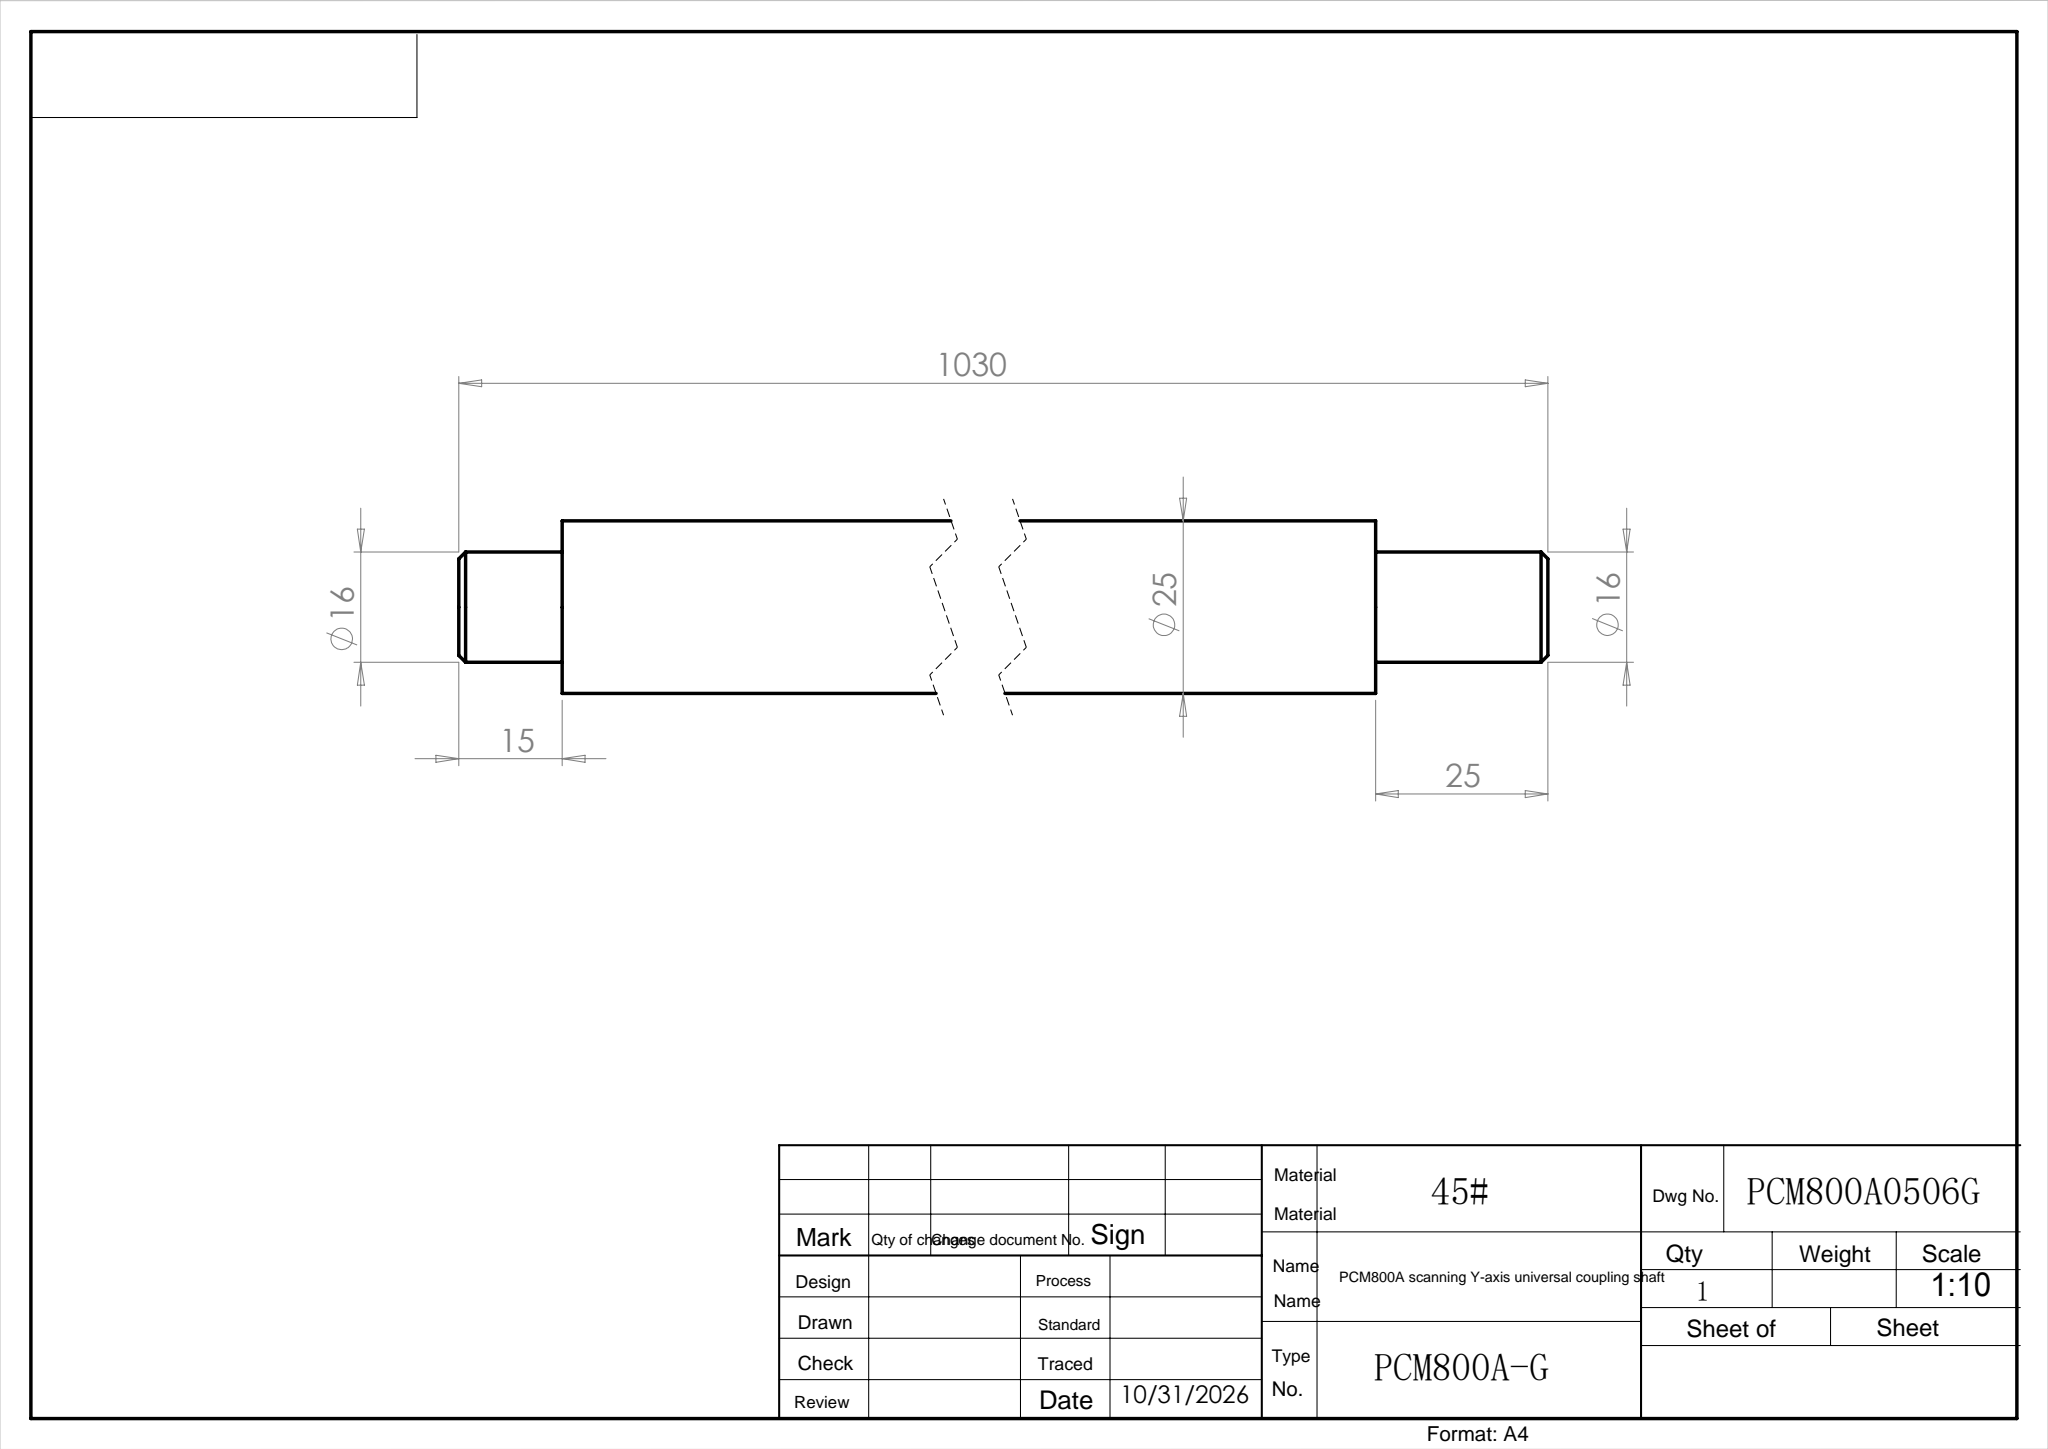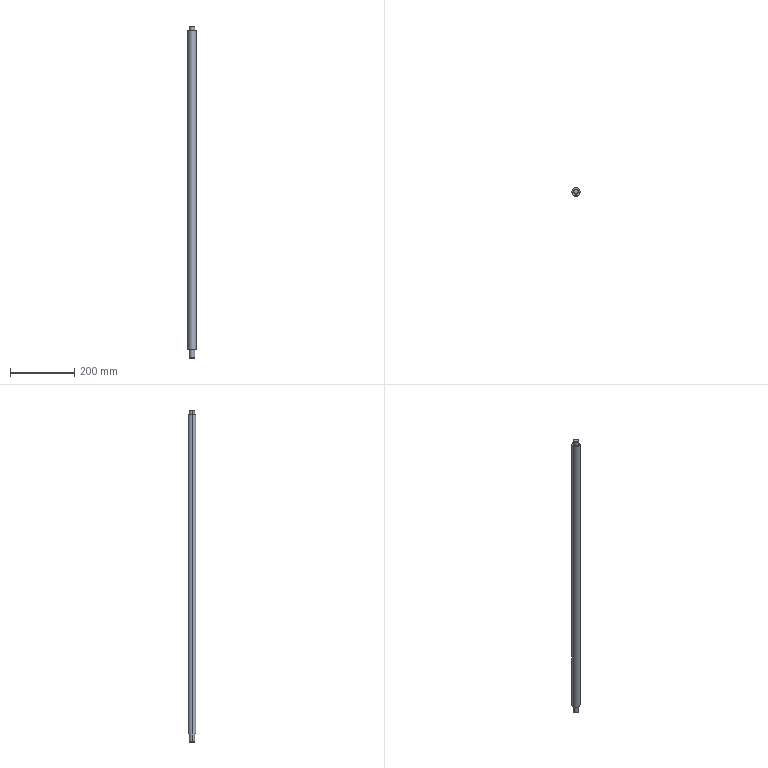Part | SolidWorks | features ICE 2, Chamfer 1, Extrusion 1 | 1 solid | 14 faces | box 25 x 25 x 1030 mm | volume 493959 mm3 | cylinder 6 | cone 4 | plane 4 | commonest cylinder face diameters 16 x4 25 x2
STEP:
#1=CARTESIAN_POINT('',(-7.,0.,-25.));
#2=VERTEX_POINT('',#1);
#3=CARTESIAN_POINT('',(7.,0.,-25.));
#4=VERTEX_POINT('',#3);
#5=CARTESIAN_POINT('',(0.,0.,-25.));
#6=DIRECTION('',(0.,0.,-1.));
#7=DIRECTION('',(-1.,0.,0.));
#8=AXIS2_PLACEMENT_3D('',#5,#6,#7);
#9=CIRCLE('',#8,7.);
#10=EDGE_CURVE('',#2,#4,#9,.T.);
#11=ORIENTED_EDGE('',*,*,#10,.F.);
#12=CARTESIAN_POINT('',(-8.,0.,-24.));
#13=VERTEX_POINT('',#12);
#14=CARTESIAN_POINT('',(-7.,0.,-25.));
#15=DIRECTION('',(-0.7071,0.,0.7071));
#16=VECTOR('',#15,1000.);
#17=LINE('',#14,#16);
#18=EDGE_CURVE('',#2,#13,#17,.T.);
#19=ORIENTED_EDGE('',*,*,#18,.T.);
#20=CARTESIAN_POINT('',(8.,0.,-24.));
#21=VERTEX_POINT('',#20);
#22=CARTESIAN_POINT('',(0.,0.,-24.));
#23=DIRECTION('',(0.,0.,1.));
#24=DIRECTION('',(-1.,0.,0.));
#25=AXIS2_PLACEMENT_3D('',#22,#23,#24);
#26=CIRCLE('',#25,8.);
#27=EDGE_CURVE('',#21,#13,#26,.T.);
#28=ORIENTED_EDGE('',*,*,#27,.F.);
#29=CARTESIAN_POINT('',(7.,0.,-25.));
#30=DIRECTION('',(0.7071,0.,0.7071));
#31=VECTOR('',#30,1000.);
#32=LINE('',#29,#31);
#33=EDGE_CURVE('',#4,#21,#32,.T.);
#34=ORIENTED_EDGE('',*,*,#33,.F.);
#35=EDGE_LOOP('',(#11,#19,#28,#34));
#36=FACE_OUTER_BOUND('',#35,.T.);
#37=CARTESIAN_POINT('',(0.,0.,-25.));
#38=DIRECTION('',(0.,0.,1.));
#39=DIRECTION('',(1.,0.,0.));
#40=AXIS2_PLACEMENT_3D('',#37,#38,#39);
#41=CONICAL_SURFACE('',#40,7.,0.7854);
#42=ADVANCED_FACE('',(#36),#41,.T.);
#43=CARTESIAN_POINT('',(7.,0.,1005.));
#44=VERTEX_POINT('',#43);
#45=CARTESIAN_POINT('',(-7.,0.,1005.));
#46=VERTEX_POINT('',#45);
#47=CARTESIAN_POINT('',(0.,0.,1005.));
#48=DIRECTION('',(0.,0.,1.));
#49=DIRECTION('',(1.,0.,0.));
#50=AXIS2_PLACEMENT_3D('',#47,#48,#49);
#51=CIRCLE('',#50,7.);
#52=EDGE_CURVE('',#44,#46,#51,.T.);
#53=ORIENTED_EDGE('',*,*,#52,.F.);
#54=CARTESIAN_POINT('',(8.,0.,1004.));
#55=VERTEX_POINT('',#54);
#56=CARTESIAN_POINT('',(7.,0.,1005.));
#57=DIRECTION('',(0.7071,0.,-0.7071));
#58=VECTOR('',#57,1000.);
#59=LINE('',#56,#58);
#60=EDGE_CURVE('',#44,#55,#59,.T.);
#61=ORIENTED_EDGE('',*,*,#60,.T.);
#62=CARTESIAN_POINT('',(-8.,0.,1004.));
#63=VERTEX_POINT('',#62);
#64=CARTESIAN_POINT('',(0.,0.,1004.));
#65=DIRECTION('',(0.,0.,-1.));
#66=DIRECTION('',(1.,0.,0.));
#67=AXIS2_PLACEMENT_3D('',#64,#65,#66);
#68=CIRCLE('',#67,8.);
#69=EDGE_CURVE('',#63,#55,#68,.T.);
#70=ORIENTED_EDGE('',*,*,#69,.F.);
#71=CARTESIAN_POINT('',(-7.,0.,1005.));
#72=DIRECTION('',(-0.7071,0.,-0.7071));
#73=VECTOR('',#72,1000.);
#74=LINE('',#71,#73);
#75=EDGE_CURVE('',#46,#63,#74,.T.);
#76=ORIENTED_EDGE('',*,*,#75,.F.);
#77=EDGE_LOOP('',(#53,#61,#70,#76));
#78=FACE_OUTER_BOUND('',#77,.T.);
#79=CARTESIAN_POINT('',(0.,0.,1005.));
#80=DIRECTION('',(0.,0.,-1.));
#81=DIRECTION('',(-1.,0.,0.));
#82=AXIS2_PLACEMENT_3D('',#79,#80,#81);
#83=CONICAL_SURFACE('',#82,7.,0.7854);
#84=ADVANCED_FACE('',(#78),#83,.T.);
#85=ORIENTED_EDGE('',*,*,#27,.T.);
#86=CARTESIAN_POINT('',(-8.,0.,0.));
#87=VERTEX_POINT('',#86);
#88=CARTESIAN_POINT('',(-8.,0.,-25.));
#89=DIRECTION('',(0.,0.,1.));
#90=VECTOR('',#89,1000.);
#91=LINE('',#88,#90);
#92=EDGE_CURVE('',#13,#87,#91,.T.);
#93=ORIENTED_EDGE('',*,*,#92,.T.);
#94=CARTESIAN_POINT('',(8.,0.,0.));
#95=VERTEX_POINT('',#94);
#96=CARTESIAN_POINT('',(0.,0.,0.));
#97=DIRECTION('',(0.,0.,-1.));
#98=DIRECTION('',(1.,0.,0.));
#99=AXIS2_PLACEMENT_3D('',#96,#97,#98);
#100=CIRCLE('',#99,8.);
#101=EDGE_CURVE('',#87,#95,#100,.T.);
#102=ORIENTED_EDGE('',*,*,#101,.T.);
#103=CARTESIAN_POINT('',(8.,0.,-25.));
#104=DIRECTION('',(0.,0.,1.));
#105=VECTOR('',#104,1000.);
#106=LINE('',#103,#105);
#107=EDGE_CURVE('',#21,#95,#106,.T.);
#108=ORIENTED_EDGE('',*,*,#107,.F.);
#109=EDGE_LOOP('',(#85,#93,#102,#108));
#110=FACE_OUTER_BOUND('',#109,.T.);
#111=CARTESIAN_POINT('',(0.,0.,-25.));
#112=DIRECTION('',(0.,0.,1.));
#113=DIRECTION('',(1.,0.,0.));
#114=AXIS2_PLACEMENT_3D('',#111,#112,#113);
#115=CYLINDRICAL_SURFACE('',#114,8.);
#116=ADVANCED_FACE('',(#110),#115,.T.);
#117=ORIENTED_EDGE('',*,*,#69,.T.);
#118=CARTESIAN_POINT('',(8.,0.,990.));
#119=VERTEX_POINT('',#118);
#120=CARTESIAN_POINT('',(8.,0.,1005.));
#121=DIRECTION('',(0.,0.,-1.));
#122=VECTOR('',#121,1000.);
#123=LINE('',#120,#122);
#124=EDGE_CURVE('',#55,#119,#123,.T.);
#125=ORIENTED_EDGE('',*,*,#124,.T.);
#126=CARTESIAN_POINT('',(-8.,0.,990.));
#127=VERTEX_POINT('',#126);
#128=CARTESIAN_POINT('',(0.,0.,990.));
#129=DIRECTION('',(0.,0.,1.));
#130=DIRECTION('',(1.,0.,0.));
#131=AXIS2_PLACEMENT_3D('',#128,#129,#130);
#132=CIRCLE('',#131,8.);
#133=EDGE_CURVE('',#119,#127,#132,.T.);
#134=ORIENTED_EDGE('',*,*,#133,.T.);
#135=CARTESIAN_POINT('',(-8.,0.,1005.));
#136=DIRECTION('',(0.,0.,-1.));
#137=VECTOR('',#136,1000.);
#138=LINE('',#135,#137);
#139=EDGE_CURVE('',#63,#127,#138,.T.);
#140=ORIENTED_EDGE('',*,*,#139,.F.);
#141=EDGE_LOOP('',(#117,#125,#134,#140));
#142=FACE_OUTER_BOUND('',#141,.T.);
#143=CARTESIAN_POINT('',(0.,0.,1005.));
#144=DIRECTION('',(0.,0.,-1.));
#145=DIRECTION('',(-1.,0.,0.));
#146=AXIS2_PLACEMENT_3D('',#143,#144,#145);
#147=CYLINDRICAL_SURFACE('',#146,8.);
#148=ADVANCED_FACE('',(#142),#147,.T.);
#149=CARTESIAN_POINT('',(12.5,0.,990.));
#150=VERTEX_POINT('',#149);
#151=CARTESIAN_POINT('',(-12.5,0.,990.));
#152=VERTEX_POINT('',#151);
#153=CARTESIAN_POINT('',(0.,0.,990.));
#154=DIRECTION('',(0.,0.,1.));
#155=DIRECTION('',(1.,0.,0.));
#156=AXIS2_PLACEMENT_3D('',#153,#154,#155);
#157=CIRCLE('',#156,12.5);
#158=EDGE_CURVE('',#150,#152,#157,.T.);
#159=ORIENTED_EDGE('',*,*,#158,.F.);
#160=CARTESIAN_POINT('',(12.5,0.,0.));
#161=VERTEX_POINT('',#160);
#162=CARTESIAN_POINT('',(12.5,0.,990.));
#163=DIRECTION('',(0.,0.,-1.));
#164=VECTOR('',#163,1000.);
#165=LINE('',#162,#164);
#166=EDGE_CURVE('',#150,#161,#165,.T.);
#167=ORIENTED_EDGE('',*,*,#166,.T.);
#168=CARTESIAN_POINT('',(-12.5,0.,0.));
#169=VERTEX_POINT('',#168);
#170=CARTESIAN_POINT('',(0.,0.,0.));
#171=DIRECTION('',(0.,0.,1.));
#172=DIRECTION('',(1.,0.,0.));
#173=AXIS2_PLACEMENT_3D('',#170,#171,#172);
#174=CIRCLE('',#173,12.5);
#175=EDGE_CURVE('',#161,#169,#174,.T.);
#176=ORIENTED_EDGE('',*,*,#175,.T.);
#177=CARTESIAN_POINT('',(-12.5,0.,990.));
#178=DIRECTION('',(0.,0.,-1.));
#179=VECTOR('',#178,1000.);
#180=LINE('',#177,#179);
#181=EDGE_CURVE('',#152,#169,#180,.T.);
#182=ORIENTED_EDGE('',*,*,#181,.F.);
#183=EDGE_LOOP('',(#159,#167,#176,#182));
#184=FACE_OUTER_BOUND('',#183,.T.);
#185=CARTESIAN_POINT('',(0.,0.,990.));
#186=DIRECTION('',(0.,0.,-1.));
#187=DIRECTION('',(-1.,0.,0.));
#188=AXIS2_PLACEMENT_3D('',#185,#186,#187);
#189=CYLINDRICAL_SURFACE('',#188,12.5);
#190=ADVANCED_FACE('',(#184),#189,.T.);
#191=CARTESIAN_POINT('',(0.,0.,0.));
#192=DIRECTION('',(0.,0.,1.));
#193=DIRECTION('',(1.,0.,0.));
#194=AXIS2_PLACEMENT_3D('',#191,#192,#193);
#195=CIRCLE('',#194,12.5);
#196=EDGE_CURVE('',#169,#161,#195,.T.);
#197=ORIENTED_EDGE('',*,*,#196,.F.);
#198=ORIENTED_EDGE('',*,*,#175,.F.);
#199=EDGE_LOOP('',(#197,#198));
#200=FACE_OUTER_BOUND('',#199,.T.);
#201=CARTESIAN_POINT('',(0.,0.,0.));
#202=DIRECTION('',(0.,0.,-1.));
#203=DIRECTION('',(1.,0.,0.));
#204=AXIS2_PLACEMENT_3D('',#201,#202,#203);
#205=CIRCLE('',#204,8.);
#206=EDGE_CURVE('',#95,#87,#205,.T.);
#207=ORIENTED_EDGE('',*,*,#206,.F.);
#208=ORIENTED_EDGE('',*,*,#101,.F.);
#209=EDGE_LOOP('',(#207,#208));
#210=FACE_BOUND('',#209,.T.);
#211=CARTESIAN_POINT('',(0.,0.,0.));
#212=DIRECTION('',(0.,0.,1.));
#213=DIRECTION('',(1.,0.,0.));
#214=AXIS2_PLACEMENT_3D('',#211,#212,#213);
#215=PLANE('',#214);
#216=ADVANCED_FACE('',(#200,#210),#215,.F.);
#217=CARTESIAN_POINT('',(0.,0.,990.));
#218=DIRECTION('',(0.,0.,1.));
#219=DIRECTION('',(1.,0.,0.));
#220=AXIS2_PLACEMENT_3D('',#217,#218,#219);
#221=CIRCLE('',#220,12.5);
#222=EDGE_CURVE('',#152,#150,#221,.T.);
#223=ORIENTED_EDGE('',*,*,#222,.T.);
#224=ORIENTED_EDGE('',*,*,#158,.T.);
#225=EDGE_LOOP('',(#223,#224));
#226=FACE_OUTER_BOUND('',#225,.T.);
#227=CARTESIAN_POINT('',(0.,0.,990.));
#228=DIRECTION('',(0.,0.,1.));
#229=DIRECTION('',(1.,0.,0.));
#230=AXIS2_PLACEMENT_3D('',#227,#228,#229);
#231=CIRCLE('',#230,8.);
#232=EDGE_CURVE('',#127,#119,#231,.T.);
#233=ORIENTED_EDGE('',*,*,#232,.F.);
#234=ORIENTED_EDGE('',*,*,#133,.F.);
#235=EDGE_LOOP('',(#233,#234));
#236=FACE_BOUND('',#235,.T.);
#237=CARTESIAN_POINT('',(0.,0.,990.));
#238=DIRECTION('',(0.,0.,1.));
#239=DIRECTION('',(1.,0.,0.));
#240=AXIS2_PLACEMENT_3D('',#237,#238,#239);
#241=PLANE('',#240);
#242=ADVANCED_FACE('',(#226,#236),#241,.T.);
#243=ORIENTED_EDGE('',*,*,#166,.F.);
#244=ORIENTED_EDGE('',*,*,#222,.F.);
#245=ORIENTED_EDGE('',*,*,#181,.T.);
#246=ORIENTED_EDGE('',*,*,#196,.T.);
#247=EDGE_LOOP('',(#243,#244,#245,#246));
#248=FACE_OUTER_BOUND('',#247,.T.);
#249=CARTESIAN_POINT('',(0.,0.,990.));
#250=DIRECTION('',(0.,0.,-1.));
#251=DIRECTION('',(-1.,0.,0.));
#252=AXIS2_PLACEMENT_3D('',#249,#250,#251);
#253=CYLINDRICAL_SURFACE('',#252,12.5);
#254=ADVANCED_FACE('',(#248),#253,.T.);
#255=ORIENTED_EDGE('',*,*,#124,.F.);
#256=CARTESIAN_POINT('',(0.,0.,1004.));
#257=DIRECTION('',(0.,0.,-1.));
#258=DIRECTION('',(1.,0.,0.));
#259=AXIS2_PLACEMENT_3D('',#256,#257,#258);
#260=CIRCLE('',#259,8.);
#261=EDGE_CURVE('',#55,#63,#260,.T.);
#262=ORIENTED_EDGE('',*,*,#261,.T.);
#263=ORIENTED_EDGE('',*,*,#139,.T.);
#264=ORIENTED_EDGE('',*,*,#232,.T.);
#265=EDGE_LOOP('',(#255,#262,#263,#264));
#266=FACE_OUTER_BOUND('',#265,.T.);
#267=CARTESIAN_POINT('',(0.,0.,1005.));
#268=DIRECTION('',(0.,0.,-1.));
#269=DIRECTION('',(-1.,0.,0.));
#270=AXIS2_PLACEMENT_3D('',#267,#268,#269);
#271=CYLINDRICAL_SURFACE('',#270,8.);
#272=ADVANCED_FACE('',(#266),#271,.T.);
#273=CARTESIAN_POINT('',(0.,0.,1005.));
#274=DIRECTION('',(0.,0.,1.));
#275=DIRECTION('',(1.,0.,0.));
#276=AXIS2_PLACEMENT_3D('',#273,#274,#275);
#277=CIRCLE('',#276,7.);
#278=EDGE_CURVE('',#46,#44,#277,.T.);
#279=ORIENTED_EDGE('',*,*,#278,.T.);
#280=ORIENTED_EDGE('',*,*,#52,.T.);
#281=EDGE_LOOP('',(#279,#280));
#282=FACE_OUTER_BOUND('',#281,.T.);
#283=CARTESIAN_POINT('',(0.,0.,1005.));
#284=DIRECTION('',(0.,0.,1.));
#285=DIRECTION('',(1.,0.,0.));
#286=AXIS2_PLACEMENT_3D('',#283,#284,#285);
#287=PLANE('',#286);
#288=ADVANCED_FACE('',(#282),#287,.T.);
#289=ORIENTED_EDGE('',*,*,#92,.F.);
#290=CARTESIAN_POINT('',(0.,0.,-24.));
#291=DIRECTION('',(0.,0.,1.));
#292=DIRECTION('',(-1.,0.,0.));
#293=AXIS2_PLACEMENT_3D('',#290,#291,#292);
#294=CIRCLE('',#293,8.);
#295=EDGE_CURVE('',#13,#21,#294,.T.);
#296=ORIENTED_EDGE('',*,*,#295,.T.);
#297=ORIENTED_EDGE('',*,*,#107,.T.);
#298=ORIENTED_EDGE('',*,*,#206,.T.);
#299=EDGE_LOOP('',(#289,#296,#297,#298));
#300=FACE_OUTER_BOUND('',#299,.T.);
#301=CARTESIAN_POINT('',(0.,0.,-25.));
#302=DIRECTION('',(0.,0.,1.));
#303=DIRECTION('',(1.,0.,0.));
#304=AXIS2_PLACEMENT_3D('',#301,#302,#303);
#305=CYLINDRICAL_SURFACE('',#304,8.);
#306=ADVANCED_FACE('',(#300),#305,.T.);
#307=CARTESIAN_POINT('',(0.,0.,-25.));
#308=DIRECTION('',(0.,0.,-1.));
#309=DIRECTION('',(-1.,0.,0.));
#310=AXIS2_PLACEMENT_3D('',#307,#308,#309);
#311=CIRCLE('',#310,7.);
#312=EDGE_CURVE('',#4,#2,#311,.T.);
#313=ORIENTED_EDGE('',*,*,#312,.T.);
#314=ORIENTED_EDGE('',*,*,#10,.T.);
#315=EDGE_LOOP('',(#313,#314));
#316=FACE_OUTER_BOUND('',#315,.T.);
#317=CARTESIAN_POINT('',(0.,0.,-25.));
#318=DIRECTION('',(0.,0.,-1.));
#319=DIRECTION('',(-1.,0.,0.));
#320=AXIS2_PLACEMENT_3D('',#317,#318,#319);
#321=PLANE('',#320);
#322=ADVANCED_FACE('',(#316),#321,.T.);
#323=ORIENTED_EDGE('',*,*,#60,.F.);
#324=ORIENTED_EDGE('',*,*,#278,.F.);
#325=ORIENTED_EDGE('',*,*,#75,.T.);
#326=ORIENTED_EDGE('',*,*,#261,.F.);
#327=EDGE_LOOP('',(#323,#324,#325,#326));
#328=FACE_OUTER_BOUND('',#327,.T.);
#329=CARTESIAN_POINT('',(0.,0.,1005.));
#330=DIRECTION('',(0.,0.,-1.));
#331=DIRECTION('',(-1.,0.,0.));
#332=AXIS2_PLACEMENT_3D('',#329,#330,#331);
#333=CONICAL_SURFACE('',#332,7.,0.7854);
#334=ADVANCED_FACE('',(#328),#333,.T.);
#335=ORIENTED_EDGE('',*,*,#18,.F.);
#336=ORIENTED_EDGE('',*,*,#312,.F.);
#337=ORIENTED_EDGE('',*,*,#33,.T.);
#338=ORIENTED_EDGE('',*,*,#295,.F.);
#339=EDGE_LOOP('',(#335,#336,#337,#338));
#340=FACE_OUTER_BOUND('',#339,.T.);
#341=CARTESIAN_POINT('',(0.,0.,-25.));
#342=DIRECTION('',(0.,0.,1.));
#343=DIRECTION('',(1.,0.,0.));
#344=AXIS2_PLACEMENT_3D('',#341,#342,#343);
#345=CONICAL_SURFACE('',#344,7.,0.7854);
#346=ADVANCED_FACE('',(#340),#345,.T.);
#347=CLOSED_SHELL('',(#42,#84,#116,#148,#190,#216,#242,#254,#272,#288,#306,#322,#334,#346));
#348=MANIFOLD_SOLID_BREP('',#347);
#349=CARTESIAN_POINT('',(0.,0.,0.));
#350=DIRECTION('',(0.,0.,1.));
#351=DIRECTION('',(1.,0.,0.));
#352=AXIS2_PLACEMENT_3D('',#349,#350,#351);
#353=(LENGTH_UNIT()NAMED_UNIT(*)SI_UNIT(.MILLI.,.METRE.));
#354=UNCERTAINTY_MEASURE_WITH_UNIT(LENGTH_MEASURE(0.00001),#353,'','');
#355=(NAMED_UNIT(*)PLANE_ANGLE_UNIT()SI_UNIT($,.RADIAN.));
#356=(NAMED_UNIT(*)SI_UNIT($,.STERADIAN.)SOLID_ANGLE_UNIT());
#357=(GEOMETRIC_REPRESENTATION_CONTEXT(3)GLOBAL_UNCERTAINTY_ASSIGNED_CONTEXT((#354))GLOBAL_UNIT_ASSIGNED_CONTEXT((#353,#355,#356))REPRESENTATION_CONTEXT('',''));
#358=ADVANCED_BREP_SHAPE_REPRESENTATION('',(#348,#352),#357);